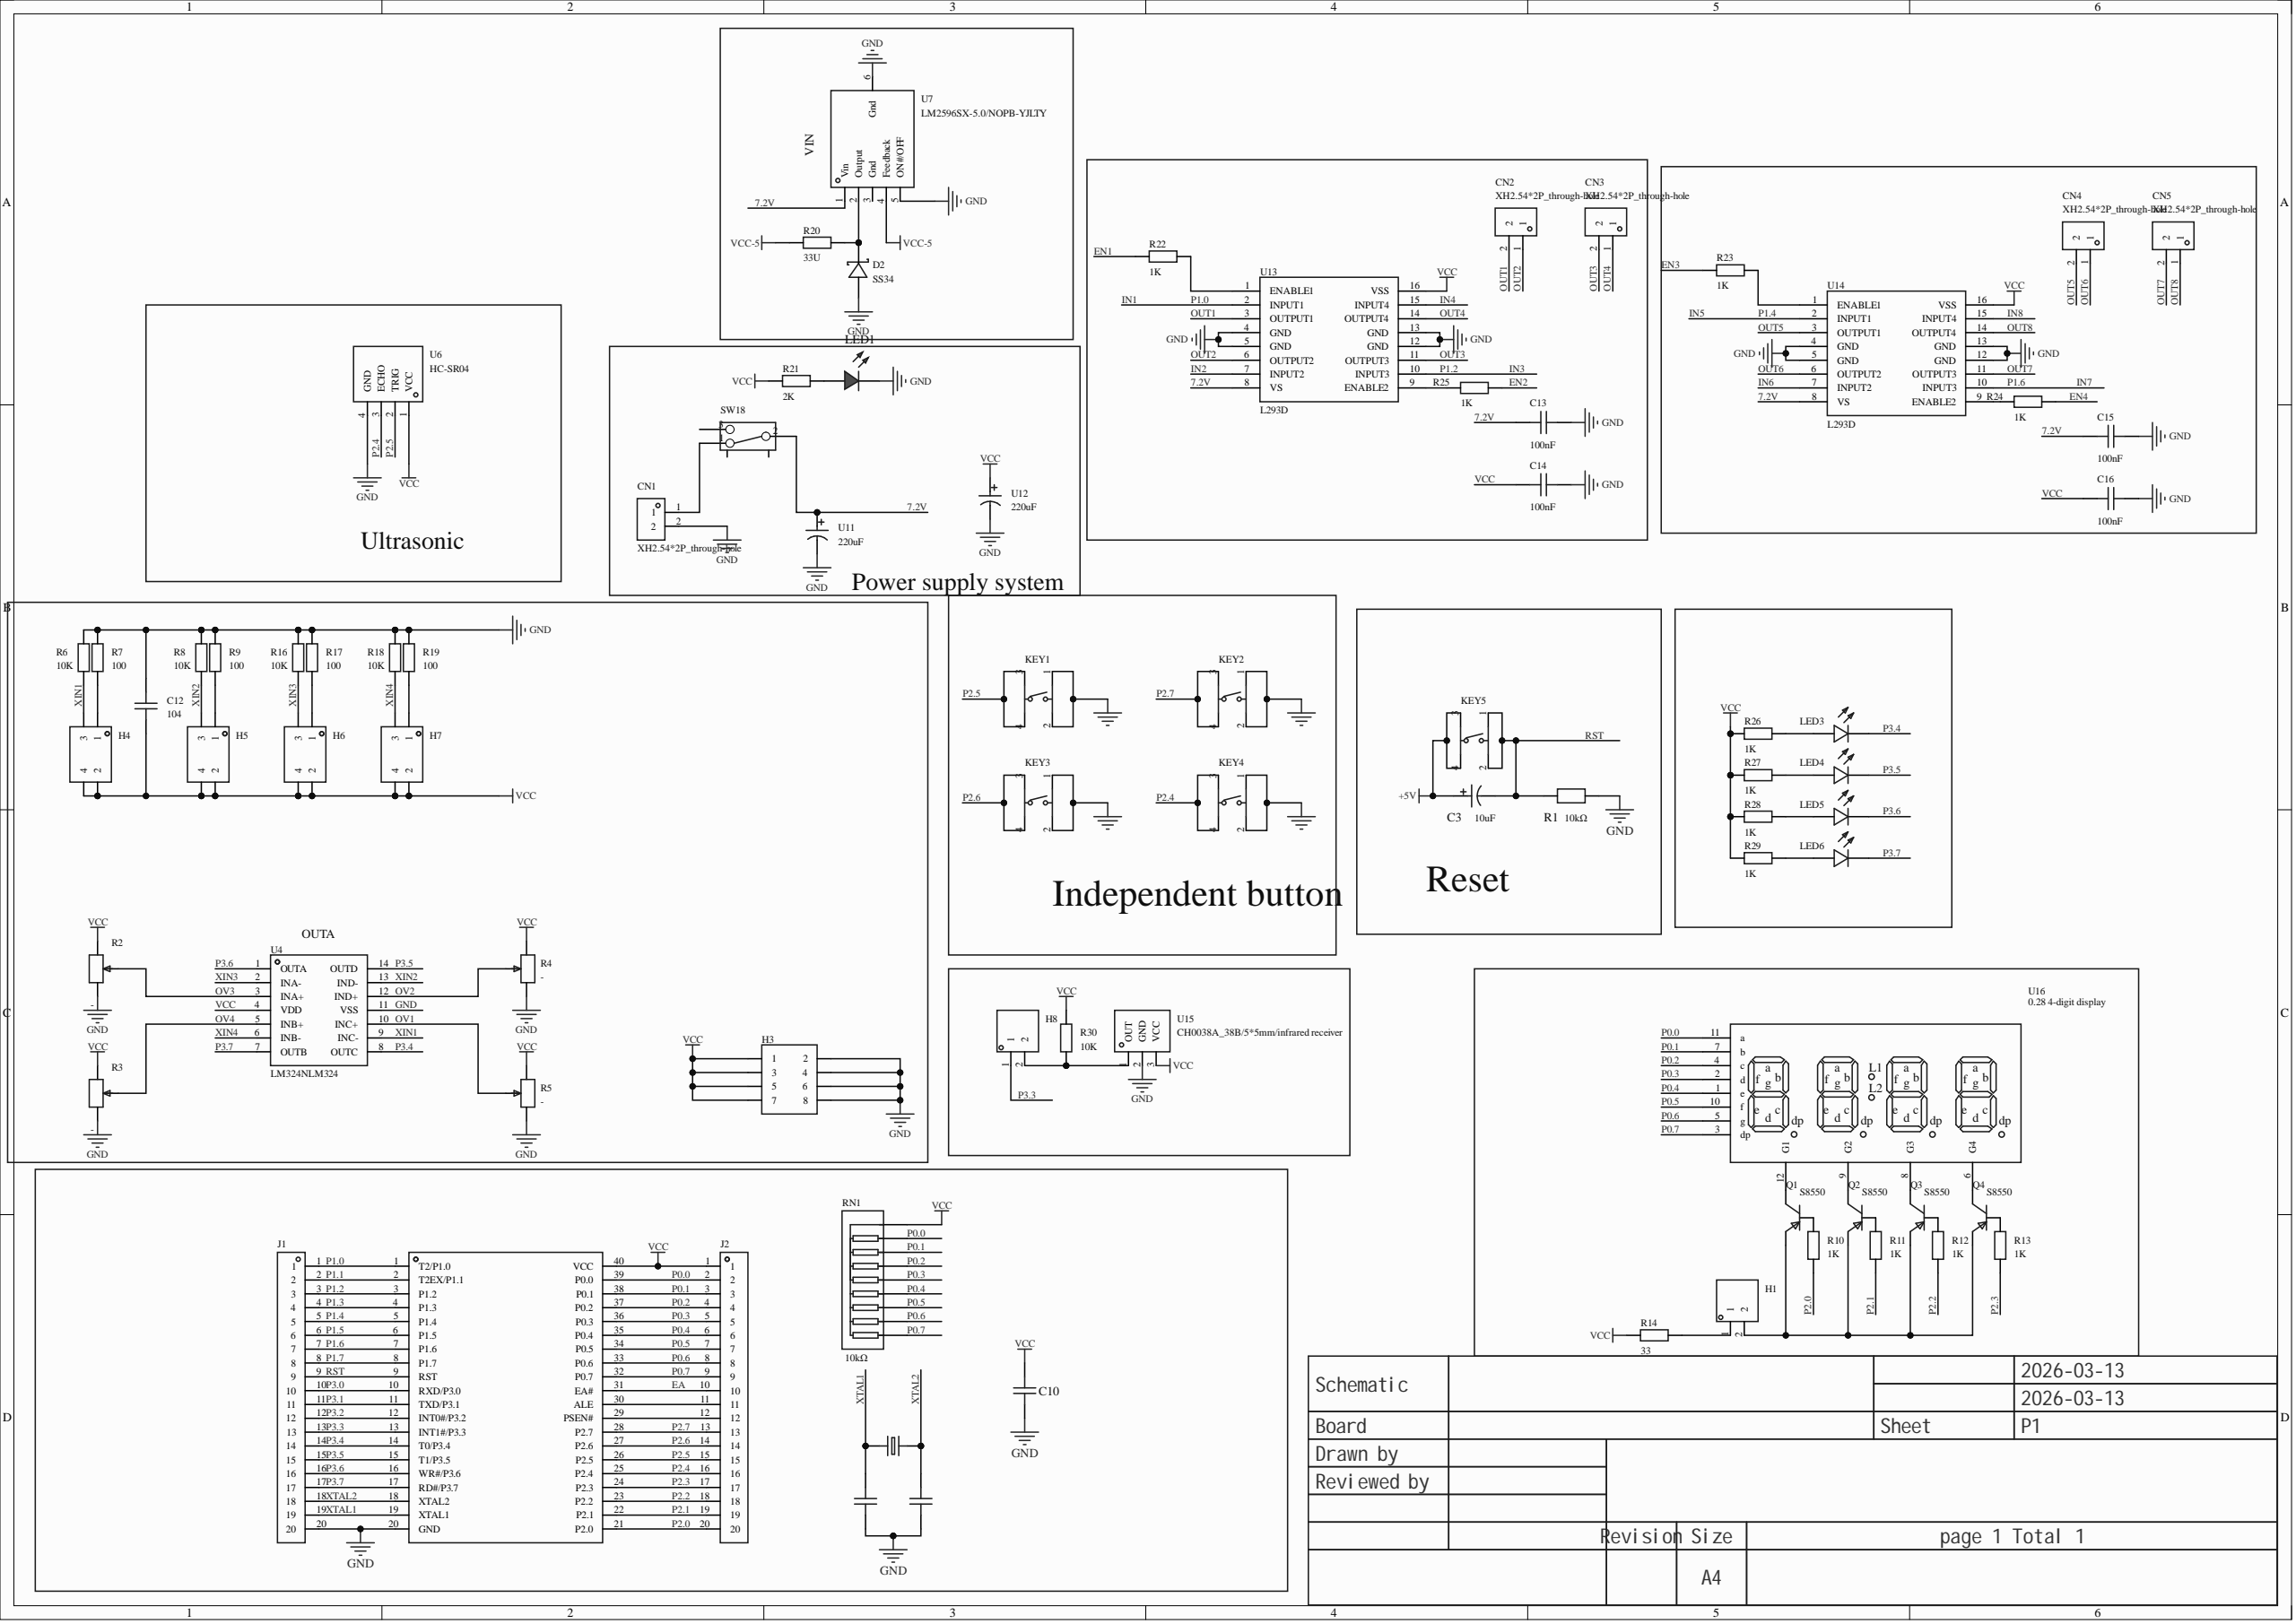Circuit board | Altium Designer | 80 parts | 85 nets
Bill of materials:
Comment,Description,Designator,Footprint,LibRef,Quantity
"","Capacitance:33pF;Tolerance:±5%;Rated voltage:50V;Temperature coefficient:NP0;Lead pitch:5.08mm;Body diameter:4.7mm;Body thickness:2.2mm;","C1, C2","CAP-TH_L5.0-W2.5-P5.08-D0.7","CC1H330JC74DCH4B10MN","2"
"","Capacitance:10uF;Tolerance:±20%;Rated voltage:50V;Body diameter:5mm;Body length:11mm;Lead pitch:2mm;Operating life:1000hrs@105;","C3","CAP-TH_BD5.0-P2.00-D0.8-FD","KM106M050D11RR0VH2FP0","1"
"","Capacitance:100nF;Tolerance:±20%;Rated voltage:50V;Temperature coefficient:Y5V;Lead pitch:5.08mm;Body diameter:6mm;Body thickness:2.2mm;","C10","CAP-TH_L5.0-W2.5-P5.00-D1.0","CC1H104MC1FD3F6C10MF","1"
"104","","C12","C0603","CAP_0603","1"
"100nF","","C13, C14, C15, C16","C0603","CAP_0603","4"
"XH2.54*2P_through-hole","","CN1, CN2, CN3, CN4, CN5","CONN-TH_2P-P2.50-XH2.54-2P","XH2.54*2P_直插","5"
"SS34","","D2","SMA_L4.3-W2.6-LS5.0-RD","SS34","1"
"","","H1, H8","HDR-TH_2P-P2.54-V-M-1","HDR-M_2.54_1x2P","2"
"","","H3","HDR-TH_8P-P2.54-V-F-R2-C4-S2.54-1","HDR-F_2.54_2x4","1"
"","","H4, H5, H6, H7","HDR-TH_4P-P2.54-V-F-R2-C2-S2.54","HDR-F_2.54_2x2","4"
"","Pitch:2.54mm;Total pin count:20;Rows:1;Pin structure:-;Row spacing:-;Mounting type:through-hole;Round/square pin:-;Rated current:-;Rated voltage:-;Mating pin length:-;Plastic height:-;Contact material:brass;Contact plating:-;Colour:black;","J1, J2","HDR-TH_20P-P2.54-V-M-1","2.54-1*20P直针","2"
"UK-B0202-G5-160","Contact current:50mA;Rated voltage (DC):12V;Insulation resistance:100MΩ;Circuit:SPST;Mounting type:through-hole;Button shape:round button;Button/cap colour:black;With lamp:no;Actuating force:160gf@±50gf;Mechanical life:100000;Operating temperature:-20~+70;Pin style:PC pin;Switch length:6mm;Switch width:6mm;Switch height:5mm;With bracket:no;","KEY1, KEY2, KEY3, KEY4, KEY5","SW-TH_4P-L6.0-W6.0-P4.50-LS6.5","UK-B0202-G5-160","5"
"","","LED1","LED_0603","LED_0603-R","1"
"","Emitted colour:red;Diode configuration:-;Lens colour:diffused red;Dominant wavelength:624nm;Peak wavelength:632nm;Colour temperature:-;Luminous flux (25):-;Test current:20mA;Forward voltage (VF):2V;Luminous intensity:80mcd;Power:60mW;Viewing angle:40°;Mounting type:-;Operating temperature:-40~+85;","LED3, LED4, LED5, LED6","LED-TH_BD3.0-P2.54-FD","204-10SURD/S530-A3-L","4"
"S8550","Transistor type:PNP;Collector current (Ic):500mA;Collector-emitter breakdown voltage (Vceo):25V;Power dissipation (Pd):300mW;DC current gain (hFE):120@50mA,1V;","Q1, Q2, Q3, Q4","SOT-23-3_L2.9-W1.6-P1.90-LS2.8-BR","S8550(RANGE:120-200)","4"
"","Resistor type:metal film resistor;Resistance:10kΩ;Tolerance:±1%;Power:250mW;Temperature coefficient:±50ppm/;Max working voltage:250V;Operating temperature range:-55~+125;","R1","RES-TH_BD2.4-L6.3-P10.30-D0.6","RN 1/4W 10K F T/B A1","1"
"-","Resistance:-;Power:-;","R2, R3, R4, R5","RES-ADJ-TH_3362P","3362P-1-103_C5047","4"
"10K","","R6, R8, R16, R18, R30","R0603","Res_0603","5"
"100","","R7, R9, R17, R19","R0603","Res_0603","4"
"1K","","R10, R11, R12, R13, R22, R23, R24, R25, R26, R27, R28, R29","R0603","Res_0603","12"
"33","","R14","R0603","Res_0603","1"
"33U","","R20","R0603","Res_0603","1"
"2K","","R21","R0603","Res_0603","1"
"","Resistance:10kΩ;Tolerance:±5%;Power per element:125mW;Temperature coefficient:±100ppm/;Number of resistors:8;Pin count:9;","RN1","RES-ARRAY-TH_9P-P2.54-D1.0","A09-103JP","1"
"","","SW18","拨动开关","拨动开关_正","1"
"","CPU core:51 series;Max CPU frequency:-;Operating voltage range:3.3V~5.5V;Internal oscillator:-;External clock frequency range:-;Program FLASH capacity:8KB;Total RAM:512Byte;EEPROM/data FLASH capacity:4KB;GPIO port count:35;ADC (units/channels/bits):-;DAC (units/channels/bits):-;(E)PWM (units/channels/bits):-;8-bit Timer count:-;16-bit Timer count:3;32-bit Timer count:-;Internal comparator count:-;U(S)ART count:1;I2C count:-;I2S count:-;(","U1","DIP-40_L52.0-W13.7-P2.54-LS15.2-BL","STC89C52RC-40I-PDIP40","1"
"LM324NLM324","","U4","SOP-14_L8.6-W3.9-P1.27-LS6.0-BL","LM324NLM324","1"
"HC-SR04","","U6","TH_HC-SR04V","HC-SR04","1"
"LM2596SX-5.0/NOPB-YJLTY","","U7","TO-263-5_L10.0-W8.4-P1.70-LS15.3-BR","LM2596SX-5.0/NOPB-YJLTY","1"
"220uF","","U11, U12","CAP-SMD_BD6.3-L6.6-W6.6-LS7.2-FD","220uF","2"
"L293D","Push-pull quad driver with diodes","U13, U14","DIP-16_L20.0-W6.4-P2.54-LS7.6-BL","L293D","2"
"CH0038A_38B/5*5mm/infrared receiver","","U15","OPTO-SMD_CH0038A_38B","CH0038A_38B/5*5mm/红外接收头","1"
"0.28 4-digit display","","U16","LED-SEG-TH_12P-L32.1-W10.0-P12.7-S7.62-BL","0.28 4位 数码管","1"
"","Crystal type:-;Frequency:-;Frequency tolerance:-;Load capacitance:-;Operating temperature:-;","X1","HC-49US_L11.5-W4.5-P4.88","TAXD12M2GLFBET2T","1"
Netlist (Protel format):
[
C1
CAP-TH_L5.0-W2.5-P5.08-D0.7




]
[
C2
CAP-TH_L5.0-W2.5-P5.08-D0.7




]
[
C3
CAP-TH_BD5.0-P2.00-D0.8-FD




]
[
C10
CAP-TH_L5.0-W2.5-P5.00-D1.0




]
[
C12
C0603
104



]
[
C13
C0603
100nF



]
[
C14
C0603
100nF



]
[
C15
C0603
100nF



]
[
C16
C0603
100nF



]
[
CN1
CONN-TH_2P-P2.50-XH2.54-2P
XH2.54*2P_through-hole



]
[
CN2
CONN-TH_2P-P2.50-XH2.54-2P
XH2.54*2P_through-hole



]
[
CN3
CONN-TH_2P-P2.50-XH2.54-2P
XH2.54*2P_through-hole



]
[
CN4
CONN-TH_2P-P2.50-XH2.54-2P
XH2.54*2P_through-hole



]
[
CN5
CONN-TH_2P-P2.50-XH2.54-2P
XH2.54*2P_through-hole



]
[
D2
SMA_L4.3-W2.6-LS5.0-RD
SS34



]
[
H1
HDR-TH_2P-P2.54-V-M-1




]
[
H3
HDR-TH_8P-P2.54-V-F-R2-C4-S2.54-1




]
[
H4
HDR-TH_4P-P2.54-V-F-R2-C2-S2.54




]
[
H5
HDR-TH_4P-P2.54-V-F-R2-C2-S2.54




]
[
H6
HDR-TH_4P-P2.54-V-F-R2-C2-S2.54




]
[
H7
HDR-TH_4P-P2.54-V-F-R2-C2-S2.54




]
[
H8
HDR-TH_2P-P2.54-V-M-1




]
[
J1
HDR-TH_20P-P2.54-V-M-1




]
[
J2
HDR-TH_20P-P2.54-V-M-1




]
[
KEY1
SW-TH_4P-L6.0-W6.0-P4.50-LS6.5
UK-B0202-G5-160



]
[
KEY2
SW-TH_4P-L6.0-W6.0-P4.50-LS6.5
UK-B0202-G5-160



]
[
KEY3
SW-TH_4P-L6.0-W6.0-P4.50-LS6.5
UK-B0202-G5-160



]
[
KEY4
SW-TH_4P-L6.0-W6.0-P4.50-LS6.5
UK-B0202-G5-160



]
[
KEY5
SW-TH_4P-L6.0-W6.0-P4.50-LS6.5
UK-B0202-G5-160



]
[
LED1
LED_0603




]
[
LED3
LED-TH_BD3.0-P2.54-FD




]
[
LED4
LED-TH_BD3.0-P2.54-FD




]
[
LED5
LED-TH_BD3.0-P2.54-FD




]
[
LED6
LED-TH_BD3.0-P2.54-FD




]
[
Q1
SOT-23-3_L2.9-W1.6-P1.90-LS2.8-BR
S8550



]
[
Q2
SOT-23-3_L2.9-W1.6-P1.90-LS2.8-BR
S8550



]
[
Q3
SOT-23-3_L2.9-W1.6-P1.90-LS2.8-BR
S8550



]
[
Q4
SOT-23-3_L2.9-W1.6-P1.90-LS2.8-BR
S8550



]
[
R1
RES-TH_BD2.4-L6.3-P10.30-D0.6




]
[
R2
RES-ADJ-TH_3362P
-



]
[
R3
RES-ADJ-TH_3362P
-



]
[
R4
RES-ADJ-TH_3362P
-



]
[
R5
RES-ADJ-TH_3362P
-



]
[
R6
R0603
10K



]
[
R7
R0603
100



]
[
R8
R0603
10K



]
[
R9
R0603
100



]
[
R10
R0603
1K



]
[
R11
R0603
1K



]
[
R12
R0603
1K



]
[
R13
R0603
1K



]
[
R14
R0603
33



]
[
R16
R0603
10K



]
[
R17
R0603
100



]
[
R18
R0603
10K



]
[
R19
R0603
100



]
[
R20
R0603
33U



]
[
R21
R0603
2K



]
[
R22
R0603
1K



]
[
R23
R0603
1K



]
[
R24
R0603
1K



]
[
R25
R0603
1K



]
[
R26
R0603
1K



]
[
R27
R0603
1K



]
[
R28
R0603
1K



]
[
R29
R0603
1K



]
[
R30
R0603
10K



]
[
RN1
RES-ARRAY-TH_9P-P2.54-D1.0




]
[
SW18
拨动开关




]
[
U1
DIP-40_L52.0-W13.7-P2.54-LS15.2-BL




]
[
U4
SOP-14_L8.6-W3.9-P1.27-LS6.0-BL
LM324NLM324



]
[
U6
TH_HC-SR04V
HC-SR04



]
[
U7
TO-263-5_L10.0-W8.4-P1.70-LS15.3-BR
LM2596SX-5.0/NOPB-YJLTY



]
[
U11
CAP-SMD_BD6.3-L6.6-W6.6-LS7.2-FD
220uF



]
[
U12
CAP-SMD_BD6.3-L6.6-W6.6-LS7.2-FD
220uF



]
[
U13
DIP-16_L20.0-W6.4-P2.54-LS7.6-BL
L293D



]
[
U14
DIP-16_L20.0-W6.4-P2.54-LS7.6-BL
L293D



]
[
U15
OPTO-SMD_CH0038A_38B
CH0038A_38B/5*5mm/infrared receiver



]
[
U16
LED-SEG-TH_12P-L32.1-W10.0-P12.7-S7.62-BL
0.28 4-digit display



]
[
X1
HC-49US_L11.5-W4.5-P4.88




]
(
XTAL2
C2-1
J1-18
U1-18
X1-1
)
(
XTAL1
C1-1
J1-19
U1-19
X1-2
)
(
XIN4
H7-3
R18-1
U4-6
)
(
XIN3
H6-3
R16-1
U4-2
)
(
XIN2
H5-3
R8-1
U4-13
)
(
XIN1
H4-3
R6-1
U4-9
)
(
VCC-5
R20-1
U7-4
)
(
VCC
C10-2
C12-1
C14-1
C16-1
H3-1
H3-3
H3-5
H3-7
H4-2
H4-4
H5-2
H5-4
H6-2
H6-4
H7-2
H7-4
J2-1
R2-1
R3-1
R4-1
R5-1
R14-1
R21-1
R26-1
R27-1
R28-1
R29-1
R30-2
RN1-1
U1-40
U4-4
U6-1
U12-1
U13-16
U14-16
U15-3
)
(
RST
C3-2
J1-9
KEY5-1
KEY5-2
R1-1
U1-9
)
(
P3.7
J1-17
LED6-2
U1-17
U4-7
)
(
P3.6
J1-16
LED5-2
U1-16
U4-1
)
(
P3.5
J1-15
LED4-2
U1-15
U4-14
)
(
P3.4
J1-14
LED3-2
U1-14
U4-8
)
(
P3.3
H8-1
J1-13
U1-13
)
(
P3.2
J1-12
U1-12
)
(
P3.1
J1-11
U1-11
)
(
P3.0
J1-10
U1-10
)
(
P2.7
J2-13
KEY2-3
KEY2-4
U1-28
)
(
P2.6
J2-14
KEY3-3
KEY3-4
U1-27
)
(
P2.5
J2-15
KEY1-3
KEY1-4
U1-26
U6-2
)
(
P2.4
J2-16
KEY4-3
KEY4-4
U1-25
U6-3
)
(
P2.3
J2-17
R13-1
U1-24
)
(
P2.2
J2-18
R12-1
U1-23
)
(
P2.1
J2-19
R11-1
U1-22
)
(
P2.0
J2-20
R10-1
U1-21
)
(
P1.7
J1-8
U1-8
)
(
P1.5
J1-6
U1-6
)
(
P1.3
J1-4
U1-4
)
(
P1.1
J1-2
U1-2
)
(
P0.7
J2-9
RN1-9
U1-32
U16-3
)
(
P0.6
J2-8
RN1-8
U1-33
U16-5
)
(
P0.5
J2-7
RN1-7
U1-34
U16-10
)
(
P0.4
J2-6
RN1-6
U1-35
U16-1
)
(
P0.3
J2-5
RN1-5
U1-36
U16-2
)
(
P0.2
J2-4
RN1-4
U1-37
U16-4
)
(
P0.1
J2-3
RN1-3
U1-38
U16-7
)
(
P0.0
J2-2
RN1-2
U1-39
U16-11
)
(
OV4
R3-2
U4-5
)
(
OV3
R2-2
U4-3
)
(
OV2
R4-2
U4-12
)
(
OV1
R5-2
U4-10
)
(
OUT8
CN5-1
U14-14
)
(
OUT7
CN5-2
U14-11
)
(
OUT6
CN4-1
U14-6
)
(
OUT5
CN4-2
U14-3
)
(
OUT4
CN3-1
U13-14
)
(
OUT3
CN3-2
U13-11
)
(
OUT2
CN2-1
U13-6
)
(
OUT1
CN2-2
U13-3
)
(
NetR25_1
R25-1
U13-9
)
(
NetR24_1
R24-1
U14-9
)
(
NetR23_2
R23-2
U14-1
)
(
NetR22_2
R22-2
U13-1
)
(
NetQ4_3
Q4-3
U16-6
)
(
NetQ4_1
Q4-1
R13-2
)
(
NetQ3_3
Q3-3
U16-8
)
(
NetQ3_1
Q3-1
R12-2
)
(
NetQ2_3
Q2-3
U16-9
)
(
NetQ2_1
Q2-1
R11-2
)
(
NetQ1_3
Q1-3
U16-12
)
(
NetQ1_1
Q1-1
R10-2
)
(
NetLED6_1
LED6-1
R29-2
)
(
NetLED5_1
LED5-1
R28-2
)
(
NetLED4_1
LED4-1
R27-2
)
(
NetLED3_1
LED3-1
R26-2
)
(
NetLED1_2
LED1-2
R21-2
)
(
NetJ2_12
J2-12
U1-29
)
(
NetJ2_11
J2-11
U1-30
)
(
NetH8_2
H8-2
R30-1
U15-1
)
(
NetH7_1
H7-1
R19-1
)
(
NetH6_1
H6-1
R17-1
)
(
NetH5_1
H5-1
R9-1
)
(
NetH4_1
H4-1
R7-1
)
(
NetH1_2
H1-2
Q1-2
Q2-2
Q3-2
Q4-2
)
(
NetH1_1
H1-1
R14-2
)
(
NetD2_1
D2-1
R20-2
U7-2
)
(
NetCN1_1
CN1-1
SW18-1
)
(
IN7
J1-7
U1-7
U14-10
)
(
IN5
J1-5
U1-5
U14-2
)
(
IN3
J1-3
U1-3
U13-10
)
(
IN1
J1-1
U1-1
U13-2
)
(
GND
C1-2
C2-2
C10-1
C12-2
C13-2
C14-2
C15-2
C16-2
CN1-2
D2-2
H3-2
H3-4
H3-6
H3-8
J1-20
KEY1-1
KEY1-2
KEY2-1
KEY2-2
KEY3-1
KEY3-2
KEY4-1
KEY4-2
LED1-1
R1-2
R2-3
R3-3
R4-3
R5-3
R6-2
R7-2
R8-2
R9-2
R16-2
R17-2
R18-2
R19-2
U1-20
U4-11
U6-4
U7-5
U7-6
U11-2
U12-2
U13-4
U13-5
U13-12
U13-13
U14-4
U14-5
U14-12
U14-13
U15-2
)
(
EA
J2-10
U1-31
)
(
+5V
C3-1
KEY5-3
KEY5-4
)
(
7.2V
C13-1
C15-1
SW18-2
U7-1
U11-1
U13-8
U14-8
)